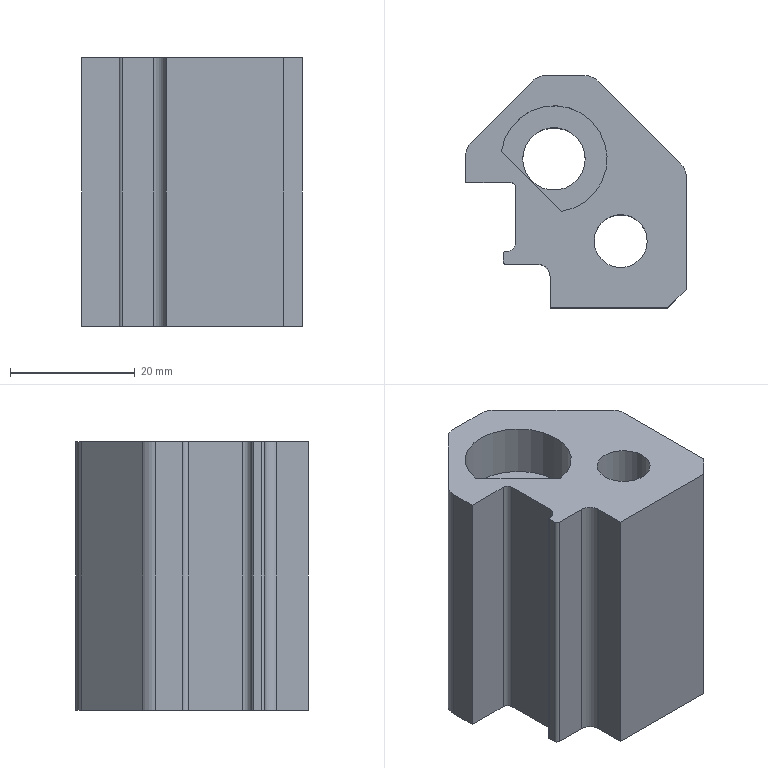Part | NX | features PH-3 2 | 1 solid | 31 faces | box 35.315 x 37.187 x 43 mm | volume 32210 mm3 | plane 18 | cylinder 13 | commonest cylinder face diameters 6 x4 0.6 x1 1 x1 2 x1 3 x1 4 x1
STEP:
#1=CARTESIAN_POINT('',(2388.447,-916.264,902.716));
#2=VERTEX_POINT('',#1);
#3=CARTESIAN_POINT('',(2398.248,-906.463,902.716));
#4=VERTEX_POINT('',#3);
#5=CARTESIAN_POINT('',(2389.755,-914.956,902.716));
#6=DIRECTION('',(-0.7071,-0.7071,0.));
#7=VECTOR('',#6,1000.);
#8=LINE('',#5,#7);
#9=EDGE_CURVE('',#2,#4,#8,.F.);
#10=ORIENTED_EDGE('',*,*,#9,.F.);
#11=CARTESIAN_POINT('',(2388.447,-916.264,945.716));
#12=VERTEX_POINT('',#11);
#13=CARTESIAN_POINT('',(2388.447,-916.264,920.716));
#14=DIRECTION('',(0.,0.,1.));
#15=VECTOR('',#14,1000.);
#16=LINE('',#13,#15);
#17=EDGE_CURVE('',#2,#12,#16,.T.);
#18=ORIENTED_EDGE('',*,*,#17,.T.);
#19=CARTESIAN_POINT('',(2398.248,-906.463,945.716));
#20=VERTEX_POINT('',#19);
#21=CARTESIAN_POINT('',(2389.755,-914.956,945.716));
#22=DIRECTION('',(0.7071,0.7071,0.));
#23=VECTOR('',#22,1000.);
#24=LINE('',#21,#23);
#25=EDGE_CURVE('',#20,#12,#24,.F.);
#26=ORIENTED_EDGE('',*,*,#25,.F.);
#27=CARTESIAN_POINT('',(2398.248,-906.463,920.716));
#28=DIRECTION('',(0.,0.,1.));
#29=VECTOR('',#28,1000.);
#30=LINE('',#27,#29);
#31=EDGE_CURVE('',#20,#4,#30,.F.);
#32=ORIENTED_EDGE('',*,*,#31,.T.);
#33=EDGE_LOOP('',(#10,#18,#26,#32));
#34=FACE_BOUND('',#33,.T.);
#35=CARTESIAN_POINT('',(2397.005,-907.706,920.716));
#36=DIRECTION('',(0.7071,-0.7071,0.));
#37=DIRECTION('',(0.,0.,1.));
#38=AXIS2_PLACEMENT_3D('',#35,#36,#37);
#39=PLANE('',#38);
#40=ADVANCED_FACE('',(#34),#39,.F.);
#41=CARTESIAN_POINT('',(2393.285,-917.695,945.716));
#42=VERTEX_POINT('',#41);
#43=CARTESIAN_POINT('',(2402.901,-927.312,945.716));
#44=VERTEX_POINT('',#43);
#45=CARTESIAN_POINT('',(2398.093,-922.503,945.716));
#46=DIRECTION('',(0.7071,-0.7071,0.));
#47=VECTOR('',#46,1000.);
#48=LINE('',#45,#47);
#49=EDGE_CURVE('',#42,#44,#48,.T.);
#50=ORIENTED_EDGE('',*,*,#49,.F.);
#51=CARTESIAN_POINT('',(2401.699,-918.897,945.716));
#52=DIRECTION('',(0.,0.,-1.));
#53=DIRECTION('',(1.,0.,0.));
#54=AXIS2_PLACEMENT_3D('',#51,#52,#53);
#55=CIRCLE('',#54,8.5);
#56=EDGE_CURVE('',#42,#44,#55,.T.);
#57=ORIENTED_EDGE('',*,*,#56,.T.);
#58=EDGE_LOOP('',(#50,#57));
#59=FACE_BOUND('',#58,.T.);
#60=CARTESIAN_POINT('',(2416.634,-932.085,945.716));
#61=VERTEX_POINT('',#60);
#62=CARTESIAN_POINT('',(2412.384,-932.085,945.716));
#63=DIRECTION('',(0.,0.,1.));
#64=DIRECTION('',(1.,0.,0.));
#65=AXIS2_PLACEMENT_3D('',#62,#63,#64);
#66=CIRCLE('',#65,4.25);
#67=EDGE_CURVE('',#61,#61,#66,.T.);
#68=ORIENTED_EDGE('',*,*,#67,.F.);
#69=EDGE_LOOP('',(#68));
#70=FACE_BOUND('',#69,.T.);
#71=ORIENTED_EDGE('',*,*,#25,.T.);
#72=CARTESIAN_POINT('',(2387.569,-918.385,945.716));
#73=VERTEX_POINT('',#72);
#74=CARTESIAN_POINT('',(2390.569,-918.385,945.716));
#75=DIRECTION('',(0.,0.,1.));
#76=DIRECTION('',(1.,0.,0.));
#77=AXIS2_PLACEMENT_3D('',#74,#75,#76);
#78=CIRCLE('',#77,3.);
#79=EDGE_CURVE('',#12,#73,#78,.T.);
#80=ORIENTED_EDGE('',*,*,#79,.T.);
#81=CARTESIAN_POINT('',(2387.569,-922.622,945.716));
#82=VERTEX_POINT('',#81);
#83=CARTESIAN_POINT('',(2387.569,-923.085,945.716));
#84=DIRECTION('',(0.,-1.,0.));
#85=VECTOR('',#84,1000.);
#86=LINE('',#83,#85);
#87=EDGE_CURVE('',#82,#73,#86,.F.);
#88=ORIENTED_EDGE('',*,*,#87,.F.);
#89=CARTESIAN_POINT('',(2394.569,-922.622,945.716));
#90=VERTEX_POINT('',#89);
#91=CARTESIAN_POINT('',(2393.069,-922.622,945.716));
#92=DIRECTION('',(-1.,0.,0.));
#93=VECTOR('',#92,1000.);
#94=LINE('',#91,#93);
#95=EDGE_CURVE('',#90,#82,#94,.T.);
#96=ORIENTED_EDGE('',*,*,#95,.F.);
#97=CARTESIAN_POINT('',(2395.569,-923.622,945.716));
#98=VERTEX_POINT('',#97);
#99=CARTESIAN_POINT('',(2394.569,-923.622,945.716));
#100=DIRECTION('',(0.,0.,1.));
#101=DIRECTION('',(1.,0.,0.));
#102=AXIS2_PLACEMENT_3D('',#99,#100,#101);
#103=CIRCLE('',#102,1.);
#104=EDGE_CURVE('',#98,#90,#103,.T.);
#105=ORIENTED_EDGE('',*,*,#104,.F.);
#106=CARTESIAN_POINT('',(2395.569,-932.272,945.716));
#107=VERTEX_POINT('',#106);
#108=CARTESIAN_POINT('',(2395.569,-923.085,945.716));
#109=DIRECTION('',(0.,-1.,0.));
#110=VECTOR('',#109,1000.);
#111=LINE('',#108,#110);
#112=EDGE_CURVE('',#107,#98,#111,.F.);
#113=ORIENTED_EDGE('',*,*,#112,.F.);
#114=CARTESIAN_POINT('',(2394.069,-933.772,945.716));
#115=VERTEX_POINT('',#114);
#116=CARTESIAN_POINT('',(2394.069,-932.272,945.716));
#117=DIRECTION('',(0.,0.,1.));
#118=DIRECTION('',(1.,0.,0.));
#119=AXIS2_PLACEMENT_3D('',#116,#117,#118);
#120=CIRCLE('',#119,1.5);
#121=EDGE_CURVE('',#115,#107,#120,.T.);
#122=ORIENTED_EDGE('',*,*,#121,.F.);
#123=CARTESIAN_POINT('',(2393.869,-933.772,945.716));
#124=VERTEX_POINT('',#123);
#125=CARTESIAN_POINT('',(2388.419,-933.772,945.716));
#126=DIRECTION('',(1.,0.,0.));
#127=VECTOR('',#126,1000.);
#128=LINE('',#125,#127);
#129=EDGE_CURVE('',#115,#124,#128,.F.);
#130=ORIENTED_EDGE('',*,*,#129,.T.);
#131=CARTESIAN_POINT('',(2393.569,-934.072,945.716));
#132=VERTEX_POINT('',#131);
#133=CARTESIAN_POINT('',(2393.869,-934.072,945.716));
#134=DIRECTION('',(0.,0.,1.));
#135=DIRECTION('',(1.,0.,0.));
#136=AXIS2_PLACEMENT_3D('',#133,#134,#135);
#137=CIRCLE('',#136,0.3);
#138=EDGE_CURVE('',#132,#124,#137,.F.);
#139=ORIENTED_EDGE('',*,*,#138,.F.);
#140=CARTESIAN_POINT('',(2393.569,-935.272,945.716));
#141=VERTEX_POINT('',#140);
#142=CARTESIAN_POINT('',(2393.569,-933.722,945.716));
#143=DIRECTION('',(0.,-1.,0.));
#144=VECTOR('',#143,1000.);
#145=LINE('',#142,#144);
#146=EDGE_CURVE('',#132,#141,#145,.T.);
#147=ORIENTED_EDGE('',*,*,#146,.T.);
#148=CARTESIAN_POINT('',(2394.069,-935.772,945.716));
#149=VERTEX_POINT('',#148);
#150=CARTESIAN_POINT('',(2394.069,-935.272,945.716));
#151=DIRECTION('',(0.,0.,-1.));
#152=DIRECTION('',(-1.,0.,0.));
#153=AXIS2_PLACEMENT_3D('',#150,#151,#152);
#154=CIRCLE('',#153,0.5);
#155=EDGE_CURVE('',#141,#149,#154,.F.);
#156=ORIENTED_EDGE('',*,*,#155,.T.);
#157=CARTESIAN_POINT('',(2399.069,-935.772,945.716));
#158=VERTEX_POINT('',#157);
#159=CARTESIAN_POINT('',(2475.144,-935.772,945.716));
#160=DIRECTION('',(1.,0.,0.));
#161=VECTOR('',#160,1000.);
#162=LINE('',#159,#161);
#163=EDGE_CURVE('',#149,#158,#162,.T.);
#164=ORIENTED_EDGE('',*,*,#163,.T.);
#165=CARTESIAN_POINT('',(2401.069,-937.772,945.716));
#166=VERTEX_POINT('',#165);
#167=CARTESIAN_POINT('',(2399.069,-937.772,945.716));
#168=DIRECTION('',(0.,0.,-1.));
#169=DIRECTION('',(-1.,0.,0.));
#170=AXIS2_PLACEMENT_3D('',#167,#168,#169);
#171=CIRCLE('',#170,2.);
#172=EDGE_CURVE('',#158,#166,#171,.T.);
#173=ORIENTED_EDGE('',*,*,#172,.T.);
#174=CARTESIAN_POINT('',(2401.069,-942.772,945.716));
#175=VERTEX_POINT('',#174);
#176=CARTESIAN_POINT('',(2401.069,-923.085,945.716));
#177=DIRECTION('',(0.,-1.,0.));
#178=VECTOR('',#177,1000.);
#179=LINE('',#176,#178);
#180=EDGE_CURVE('',#175,#166,#179,.F.);
#181=ORIENTED_EDGE('',*,*,#180,.F.);
#182=CARTESIAN_POINT('',(2419.884,-942.772,945.716));
#183=VERTEX_POINT('',#182);
#184=CARTESIAN_POINT('',(2401.644,-942.772,945.716));
#185=DIRECTION('',(1.,0.,0.));
#186=VECTOR('',#185,1000.);
#187=LINE('',#184,#186);
#188=EDGE_CURVE('',#183,#175,#187,.F.);
#189=ORIENTED_EDGE('',*,*,#188,.F.);
#190=CARTESIAN_POINT('',(2422.884,-939.772,945.716));
#191=VERTEX_POINT('',#190);
#192=CARTESIAN_POINT('',(2418.728,-943.928,945.716));
#193=DIRECTION('',(0.7071,0.7071,0.));
#194=VECTOR('',#193,1000.);
#195=LINE('',#192,#194);
#196=EDGE_CURVE('',#183,#191,#195,.T.);
#197=ORIENTED_EDGE('',*,*,#196,.T.);
#198=CARTESIAN_POINT('',(2422.884,-921.827,945.716));
#199=VERTEX_POINT('',#198);
#200=CARTESIAN_POINT('',(2422.884,-923.085,945.716));
#201=DIRECTION('',(0.,-1.,0.));
#202=VECTOR('',#201,1000.);
#203=LINE('',#200,#202);
#204=EDGE_CURVE('',#199,#191,#203,.T.);
#205=ORIENTED_EDGE('',*,*,#204,.F.);
#206=CARTESIAN_POINT('',(2422.005,-919.706,945.716));
#207=VERTEX_POINT('',#206);
#208=CARTESIAN_POINT('',(2419.884,-921.827,945.716));
#209=DIRECTION('',(0.,0.,1.));
#210=DIRECTION('',(1.,0.,0.));
#211=AXIS2_PLACEMENT_3D('',#208,#209,#210);
#212=CIRCLE('',#211,3.);
#213=EDGE_CURVE('',#199,#207,#212,.T.);
#214=ORIENTED_EDGE('',*,*,#213,.T.);
#215=CARTESIAN_POINT('',(2408.763,-906.463,945.716));
#216=VERTEX_POINT('',#215);
#217=CARTESIAN_POINT('',(2411.634,-909.335,945.716));
#218=DIRECTION('',(0.7071,-0.7071,0.));
#219=VECTOR('',#218,1000.);
#220=LINE('',#217,#219);
#221=EDGE_CURVE('',#207,#216,#220,.F.);
#222=ORIENTED_EDGE('',*,*,#221,.T.);
#223=CARTESIAN_POINT('',(2406.641,-905.585,945.716));
#224=VERTEX_POINT('',#223);
#225=CARTESIAN_POINT('',(2406.641,-908.585,945.716));
#226=DIRECTION('',(0.,0.,1.));
#227=DIRECTION('',(1.,0.,0.));
#228=AXIS2_PLACEMENT_3D('',#225,#226,#227);
#229=CIRCLE('',#228,3.);
#230=EDGE_CURVE('',#216,#224,#229,.T.);
#231=ORIENTED_EDGE('',*,*,#230,.T.);
#232=CARTESIAN_POINT('',(2400.369,-905.585,945.716));
#233=VERTEX_POINT('',#232);
#234=CARTESIAN_POINT('',(2397.884,-905.585,945.716));
#235=DIRECTION('',(1.,0.,0.));
#236=VECTOR('',#235,1000.);
#237=LINE('',#234,#236);
#238=EDGE_CURVE('',#233,#224,#237,.T.);
#239=ORIENTED_EDGE('',*,*,#238,.F.);
#240=CARTESIAN_POINT('',(2400.369,-908.585,945.716));
#241=DIRECTION('',(0.,0.,1.));
#242=DIRECTION('',(1.,0.,0.));
#243=AXIS2_PLACEMENT_3D('',#240,#241,#242);
#244=CIRCLE('',#243,3.);
#245=EDGE_CURVE('',#233,#20,#244,.T.);
#246=ORIENTED_EDGE('',*,*,#245,.T.);
#247=EDGE_LOOP('',(#71,#80,#88,#96,#105,#113,#122,#130,#139,#147,#156,#164,#173,#181,#189,#197,#205,#214,#222,#231,#239,#246));
#248=FACE_BOUND('',#247,.T.);
#249=CARTESIAN_POINT('',(2397.884,-923.085,945.716));
#250=DIRECTION('',(0.,0.,1.));
#251=DIRECTION('',(1.,0.,0.));
#252=AXIS2_PLACEMENT_3D('',#249,#250,#251);
#253=PLANE('',#252);
#254=ADVANCED_FACE('',(#59,#70,#248),#253,.T.);
#255=CARTESIAN_POINT('',(2396.699,-918.897,902.716));
#256=VERTEX_POINT('',#255);
#257=CARTESIAN_POINT('',(2401.699,-918.897,902.716));
#258=DIRECTION('',(0.,0.,-1.));
#259=DIRECTION('',(-1.,0.,0.));
#260=AXIS2_PLACEMENT_3D('',#257,#258,#259);
#261=CIRCLE('',#260,5.);
#262=EDGE_CURVE('',#256,#256,#261,.T.);
#263=ORIENTED_EDGE('',*,*,#262,.F.);
#264=EDGE_LOOP('',(#263));
#265=FACE_BOUND('',#264,.T.);
#266=CARTESIAN_POINT('',(2405.134,-932.085,902.716));
#267=VERTEX_POINT('',#266);
#268=CARTESIAN_POINT('',(2412.384,-932.085,902.716));
#269=DIRECTION('',(0.,0.,-1.));
#270=DIRECTION('',(-1.,0.,0.));
#271=AXIS2_PLACEMENT_3D('',#268,#269,#270);
#272=CIRCLE('',#271,7.25);
#273=EDGE_CURVE('',#267,#267,#272,.T.);
#274=ORIENTED_EDGE('',*,*,#273,.F.);
#275=EDGE_LOOP('',(#274));
#276=FACE_BOUND('',#275,.T.);
#277=CARTESIAN_POINT('',(2387.569,-918.385,902.716));
#278=VERTEX_POINT('',#277);
#279=CARTESIAN_POINT('',(2387.569,-922.622,902.716));
#280=VERTEX_POINT('',#279);
#281=CARTESIAN_POINT('',(2387.569,-927.947,902.716));
#282=DIRECTION('',(0.,-1.,0.));
#283=VECTOR('',#282,1000.);
#284=LINE('',#281,#283);
#285=EDGE_CURVE('',#278,#280,#284,.T.);
#286=ORIENTED_EDGE('',*,*,#285,.F.);
#287=CARTESIAN_POINT('',(2390.569,-918.385,902.716));
#288=DIRECTION('',(0.,0.,-1.));
#289=DIRECTION('',(-1.,0.,0.));
#290=AXIS2_PLACEMENT_3D('',#287,#288,#289);
#291=CIRCLE('',#290,3.);
#292=EDGE_CURVE('',#278,#2,#291,.T.);
#293=ORIENTED_EDGE('',*,*,#292,.T.);
#294=ORIENTED_EDGE('',*,*,#9,.T.);
#295=CARTESIAN_POINT('',(2400.369,-905.585,902.716));
#296=VERTEX_POINT('',#295);
#297=CARTESIAN_POINT('',(2400.369,-908.585,902.716));
#298=DIRECTION('',(0.,0.,-1.));
#299=DIRECTION('',(-1.,0.,0.));
#300=AXIS2_PLACEMENT_3D('',#297,#298,#299);
#301=CIRCLE('',#300,3.);
#302=EDGE_CURVE('',#4,#296,#301,.T.);
#303=ORIENTED_EDGE('',*,*,#302,.T.);
#304=CARTESIAN_POINT('',(2406.641,-905.585,902.716));
#305=VERTEX_POINT('',#304);
#306=CARTESIAN_POINT('',(2397.884,-905.585,902.716));
#307=DIRECTION('',(-1.,0.,0.));
#308=VECTOR('',#307,1000.);
#309=LINE('',#306,#308);
#310=EDGE_CURVE('',#305,#296,#309,.T.);
#311=ORIENTED_EDGE('',*,*,#310,.F.);
#312=CARTESIAN_POINT('',(2408.763,-906.463,902.716));
#313=VERTEX_POINT('',#312);
#314=CARTESIAN_POINT('',(2406.641,-908.585,902.716));
#315=DIRECTION('',(0.,0.,-1.));
#316=DIRECTION('',(-1.,0.,0.));
#317=AXIS2_PLACEMENT_3D('',#314,#315,#316);
#318=CIRCLE('',#317,3.);
#319=EDGE_CURVE('',#305,#313,#318,.T.);
#320=ORIENTED_EDGE('',*,*,#319,.T.);
#321=CARTESIAN_POINT('',(2422.005,-919.706,902.716));
#322=VERTEX_POINT('',#321);
#323=CARTESIAN_POINT('',(2411.634,-909.335,902.716));
#324=DIRECTION('',(-0.7071,0.7071,0.));
#325=VECTOR('',#324,1000.);
#326=LINE('',#323,#325);
#327=EDGE_CURVE('',#313,#322,#326,.F.);
#328=ORIENTED_EDGE('',*,*,#327,.T.);
#329=CARTESIAN_POINT('',(2422.884,-921.827,902.716));
#330=VERTEX_POINT('',#329);
#331=CARTESIAN_POINT('',(2419.884,-921.827,902.716));
#332=DIRECTION('',(0.,0.,-1.));
#333=DIRECTION('',(-1.,0.,0.));
#334=AXIS2_PLACEMENT_3D('',#331,#332,#333);
#335=CIRCLE('',#334,3.);
#336=EDGE_CURVE('',#322,#330,#335,.T.);
#337=ORIENTED_EDGE('',*,*,#336,.T.);
#338=CARTESIAN_POINT('',(2422.884,-939.772,902.716));
#339=VERTEX_POINT('',#338);
#340=CARTESIAN_POINT('',(2422.884,-923.085,902.716));
#341=DIRECTION('',(0.,1.,0.));
#342=VECTOR('',#341,1000.);
#343=LINE('',#340,#342);
#344=EDGE_CURVE('',#339,#330,#343,.T.);
#345=ORIENTED_EDGE('',*,*,#344,.F.);
#346=CARTESIAN_POINT('',(2419.884,-942.772,902.716));
#347=VERTEX_POINT('',#346);
#348=CARTESIAN_POINT('',(2418.728,-943.928,902.716));
#349=DIRECTION('',(-0.7071,-0.7071,0.));
#350=VECTOR('',#349,1000.);
#351=LINE('',#348,#350);
#352=EDGE_CURVE('',#339,#347,#351,.T.);
#353=ORIENTED_EDGE('',*,*,#352,.T.);
#354=CARTESIAN_POINT('',(2401.069,-942.772,902.716));
#355=VERTEX_POINT('',#354);
#356=CARTESIAN_POINT('',(2401.644,-942.772,902.716));
#357=DIRECTION('',(-1.,0.,0.));
#358=VECTOR('',#357,1000.);
#359=LINE('',#356,#358);
#360=EDGE_CURVE('',#355,#347,#359,.F.);
#361=ORIENTED_EDGE('',*,*,#360,.F.);
#362=CARTESIAN_POINT('',(2401.069,-937.772,902.716));
#363=VERTEX_POINT('',#362);
#364=CARTESIAN_POINT('',(2401.069,-945.272,902.716));
#365=DIRECTION('',(0.,-1.,0.));
#366=VECTOR('',#365,1000.);
#367=LINE('',#364,#366);
#368=EDGE_CURVE('',#363,#355,#367,.T.);
#369=ORIENTED_EDGE('',*,*,#368,.F.);
#370=CARTESIAN_POINT('',(2399.069,-935.772,902.716));
#371=VERTEX_POINT('',#370);
#372=CARTESIAN_POINT('',(2399.069,-937.772,902.716));
#373=DIRECTION('',(0.,0.,-1.));
#374=DIRECTION('',(-1.,0.,0.));
#375=AXIS2_PLACEMENT_3D('',#372,#373,#374);
#376=CIRCLE('',#375,2.);
#377=EDGE_CURVE('',#371,#363,#376,.T.);
#378=ORIENTED_EDGE('',*,*,#377,.F.);
#379=CARTESIAN_POINT('',(2394.069,-935.772,902.716));
#380=VERTEX_POINT('',#379);
#381=CARTESIAN_POINT('',(2397.884,-935.772,902.716));
#382=DIRECTION('',(1.,0.,0.));
#383=VECTOR('',#382,1000.);
#384=LINE('',#381,#383);
#385=EDGE_CURVE('',#380,#371,#384,.T.);
#386=ORIENTED_EDGE('',*,*,#385,.F.);
#387=CARTESIAN_POINT('',(2393.569,-935.272,902.716));
#388=VERTEX_POINT('',#387);
#389=CARTESIAN_POINT('',(2394.069,-935.272,902.716));
#390=DIRECTION('',(0.,0.,-1.));
#391=DIRECTION('',(-1.,0.,0.));
#392=AXIS2_PLACEMENT_3D('',#389,#390,#391);
#393=CIRCLE('',#392,0.5);
#394=EDGE_CURVE('',#380,#388,#393,.T.);
#395=ORIENTED_EDGE('',*,*,#394,.T.);
#396=CARTESIAN_POINT('',(2393.569,-934.072,902.716));
#397=VERTEX_POINT('',#396);
#398=CARTESIAN_POINT('',(2393.569,-923.085,902.716));
#399=DIRECTION('',(0.,1.,0.));
#400=VECTOR('',#399,1000.);
#401=LINE('',#398,#400);
#402=EDGE_CURVE('',#388,#397,#401,.T.);
#403=ORIENTED_EDGE('',*,*,#402,.T.);
#404=CARTESIAN_POINT('',(2393.869,-933.772,902.716));
#405=VERTEX_POINT('',#404);
#406=CARTESIAN_POINT('',(2393.869,-934.072,902.716));
#407=DIRECTION('',(0.,0.,-1.));
#408=DIRECTION('',(-1.,0.,0.));
#409=AXIS2_PLACEMENT_3D('',#406,#407,#408);
#410=CIRCLE('',#409,0.3);
#411=EDGE_CURVE('',#397,#405,#410,.T.);
#412=ORIENTED_EDGE('',*,*,#411,.T.);
#413=CARTESIAN_POINT('',(2394.069,-933.772,902.716));
#414=VERTEX_POINT('',#413);
#415=CARTESIAN_POINT('',(2397.884,-933.772,902.716));
#416=DIRECTION('',(1.,0.,0.));
#417=VECTOR('',#416,1000.);
#418=LINE('',#415,#417);
#419=EDGE_CURVE('',#405,#414,#418,.T.);
#420=ORIENTED_EDGE('',*,*,#419,.T.);
#421=CARTESIAN_POINT('',(2395.569,-932.272,902.716));
#422=VERTEX_POINT('',#421);
#423=CARTESIAN_POINT('',(2394.069,-932.272,902.716));
#424=DIRECTION('',(0.,0.,-1.));
#425=DIRECTION('',(-1.,0.,0.));
#426=AXIS2_PLACEMENT_3D('',#423,#424,#425);
#427=CIRCLE('',#426,1.5);
#428=EDGE_CURVE('',#422,#414,#427,.T.);
#429=ORIENTED_EDGE('',*,*,#428,.F.);
#430=CARTESIAN_POINT('',(2395.569,-923.622,902.716));
#431=VERTEX_POINT('',#430);
#432=CARTESIAN_POINT('',(2395.569,-923.085,902.716));
#433=DIRECTION('',(0.,1.,0.));
#434=VECTOR('',#433,1000.);
#435=LINE('',#432,#434);
#436=EDGE_CURVE('',#422,#431,#435,.T.);
#437=ORIENTED_EDGE('',*,*,#436,.T.);
#438=CARTESIAN_POINT('',(2394.569,-922.622,902.716));
#439=VERTEX_POINT('',#438);
#440=CARTESIAN_POINT('',(2394.569,-923.622,902.716));
#441=DIRECTION('',(0.,0.,-1.));
#442=DIRECTION('',(-1.,0.,0.));
#443=AXIS2_PLACEMENT_3D('',#440,#441,#442);
#444=CIRCLE('',#443,1.);
#445=EDGE_CURVE('',#439,#431,#444,.T.);
#446=ORIENTED_EDGE('',*,*,#445,.F.);
#447=CARTESIAN_POINT('',(2393.069,-922.622,902.716));
#448=DIRECTION('',(1.,0.,0.));
#449=VECTOR('',#448,1000.);
#450=LINE('',#447,#449);
#451=EDGE_CURVE('',#280,#439,#450,.T.);
#452=ORIENTED_EDGE('',*,*,#451,.F.);
#453=EDGE_LOOP('',(#286,#293,#294,#303,#311,#320,#328,#337,#345,#353,#361,#369,#378,#386,#395,#403,#412,#420,#429,#437,#446,#452));
#454=FACE_BOUND('',#453,.T.);
#455=CARTESIAN_POINT('',(2397.884,-923.085,902.716));
#456=DIRECTION('',(0.,0.,-1.));
#457=DIRECTION('',(-1.,0.,0.));
#458=AXIS2_PLACEMENT_3D('',#455,#456,#457);
#459=PLANE('',#458);
#460=ADVANCED_FACE('',(#265,#276,#454),#459,.T.);
#461=ORIENTED_EDGE('',*,*,#95,.T.);
#462=CARTESIAN_POINT('',(2387.569,-922.622,950.716));
#463=DIRECTION('',(0.,0.,-1.));
#464=VECTOR('',#463,1000.);
#465=LINE('',#462,#464);
#466=EDGE_CURVE('',#82,#280,#465,.T.);
#467=ORIENTED_EDGE('',*,*,#466,.T.);
#468=ORIENTED_EDGE('',*,*,#451,.T.);
#469=CARTESIAN_POINT('',(2394.569,-922.622,950.716));
#470=DIRECTION('',(0.,0.,-1.));
#471=VECTOR('',#470,1000.);
#472=LINE('',#469,#471);
#473=EDGE_CURVE('',#90,#439,#472,.T.);
#474=ORIENTED_EDGE('',*,*,#473,.F.);
#475=EDGE_LOOP('',(#461,#467,#468,#474));
#476=FACE_BOUND('',#475,.T.);
#477=CARTESIAN_POINT('',(2393.069,-922.622,950.716));
#478=DIRECTION('',(0.,-1.,0.));
#479=DIRECTION('',(0.,0.,1.));
#480=AXIS2_PLACEMENT_3D('',#477,#478,#479);
#481=PLANE('',#480);
#482=ADVANCED_FACE('',(#476),#481,.T.);
#483=ORIENTED_EDGE('',*,*,#310,.T.);
#484=CARTESIAN_POINT('',(2400.369,-905.585,920.716));
#485=DIRECTION('',(0.,0.,-1.));
#486=VECTOR('',#485,1000.);
#487=LINE('',#484,#486);
#488=EDGE_CURVE('',#296,#233,#487,.F.);
#489=ORIENTED_EDGE('',*,*,#488,.T.);
#490=ORIENTED_EDGE('',*,*,#238,.T.);
#491=CARTESIAN_POINT('',(2406.641,-905.585,920.716));
#492=DIRECTION('',(0.,0.,1.));
#493=VECTOR('',#492,1000.);
#494=LINE('',#491,#493);
#495=EDGE_CURVE('',#224,#305,#494,.F.);
#496=ORIENTED_EDGE('',*,*,#495,.T.);
#497=EDGE_LOOP('',(#483,#489,#490,#496));
#498=FACE_BOUND('',#497,.T.);
#499=CARTESIAN_POINT('',(2397.884,-905.585,920.716));
#500=DIRECTION('',(0.,1.,0.));
#501=DIRECTION('',(0.,0.,1.));
#502=AXIS2_PLACEMENT_3D('',#499,#500,#501);
#503=PLANE('',#502);
#504=ADVANCED_FACE('',(#498),#503,.T.);
#505=ORIENTED_EDGE('',*,*,#344,.T.);
#506=CARTESIAN_POINT('',(2422.884,-921.827,920.716));
#507=DIRECTION('',(0.,0.,-1.));
#508=VECTOR('',#507,1000.);
#509=LINE('',#506,#508);
#510=EDGE_CURVE('',#330,#199,#509,.F.);
#511=ORIENTED_EDGE('',*,*,#510,.T.);
#512=ORIENTED_EDGE('',*,*,#204,.T.);
#513=CARTESIAN_POINT('',(2422.884,-939.772,920.716));
#514=DIRECTION('',(0.,0.,-1.));
#515=VECTOR('',#514,1000.);
#516=LINE('',#513,#515);
#517=EDGE_CURVE('',#191,#339,#516,.T.);
#518=ORIENTED_EDGE('',*,*,#517,.T.);
#519=EDGE_LOOP('',(#505,#511,#512,#518));
#520=FACE_BOUND('',#519,.T.);
#521=CARTESIAN_POINT('',(2422.884,-923.085,920.716));
#522=DIRECTION('',(1.,0.,0.));
#523=DIRECTION('',(0.,0.,-1.));
#524=AXIS2_PLACEMENT_3D('',#521,#522,#523);
#525=PLANE('',#524);
#526=ADVANCED_FACE('',(#520),#525,.T.);
#527=CARTESIAN_POINT('',(2402.901,-927.312,937.416));
#528=VERTEX_POINT('',#527);
#529=CARTESIAN_POINT('',(2393.285,-917.695,937.416));
#530=VERTEX_POINT('',#529);
#531=CARTESIAN_POINT('',(2398.093,-922.503,937.416));
#532=DIRECTION('',(-0.7071,0.7071,0.));
#533=VECTOR('',#532,1000.);
#534=LINE('',#531,#533);
#535=EDGE_CURVE('',#528,#530,#534,.T.);
#536=ORIENTED_EDGE('',*,*,#535,.F.);
#537=CARTESIAN_POINT('',(2401.699,-918.897,937.416));
#538=DIRECTION('',(0.,0.,1.));
#539=DIRECTION('',(1.,0.,0.));
#540=AXIS2_PLACEMENT_3D('',#537,#538,#539);
#541=CIRCLE('',#540,8.5);
#542=EDGE_CURVE('',#528,#530,#541,.T.);
#543=ORIENTED_EDGE('',*,*,#542,.T.);
#544=EDGE_LOOP('',(#536,#543));
#545=FACE_BOUND('',#544,.T.);
#546=CARTESIAN_POINT('',(2396.699,-918.897,937.416));
#547=VERTEX_POINT('',#546);
#548=CARTESIAN_POINT('',(2401.699,-918.897,937.416));
#549=DIRECTION('',(0.,0.,-1.));
#550=DIRECTION('',(-1.,0.,0.));
#551=AXIS2_PLACEMENT_3D('',#548,#549,#550);
#552=CIRCLE('',#551,5.);
#553=EDGE_CURVE('',#547,#547,#552,.F.);
#554=ORIENTED_EDGE('',*,*,#553,.F.);
#555=EDGE_LOOP('',(#554));
#556=FACE_BOUND('',#555,.T.);
#557=CARTESIAN_POINT('',(2401.699,-918.897,937.416));
#558=DIRECTION('',(0.,0.,-1.));
#559=DIRECTION('',(-1.,0.,0.));
#560=AXIS2_PLACEMENT_3D('',#557,#558,#559);
#561=PLANE('',#560);
#562=ADVANCED_FACE('',(#545,#556),#561,.F.);
#563=CARTESIAN_POINT('',(2393.869,-933.772,874.217));
#564=DIRECTION('',(0.,0.,-1.));
#565=VECTOR('',#564,1000.);
#566=LINE('',#563,#565);
#567=EDGE_CURVE('',#124,#405,#566,.T.);
#568=ORIENTED_EDGE('',*,*,#567,.F.);
#569=ORIENTED_EDGE('',*,*,#129,.F.);
#570=CARTESIAN_POINT('',(2394.069,-933.772,950.716));
#571=DIRECTION('',(0.,0.,1.));
#572=VECTOR('',#571,1000.);
#573=LINE('',#570,#572);
#574=EDGE_CURVE('',#115,#414,#573,.F.);
#575=ORIENTED_EDGE('',*,*,#574,.T.);
#576=ORIENTED_EDGE('',*,*,#419,.F.);
#577=EDGE_LOOP('',(#568,#569,#575,#576));
#578=FACE_BOUND('',#577,.T.);
#579=CARTESIAN_POINT('',(2388.419,-933.772,950.716));
#580=DIRECTION('',(0.,1.,0.));
#581=DIRECTION('',(0.,0.,-1.));
#582=AXIS2_PLACEMENT_3D('',#579,#580,#581);
#583=PLANE('',#582);
#584=ADVANCED_FACE('',(#578),#583,.T.);
#585=ORIENTED_EDGE('',*,*,#112,.T.);
#586=CARTESIAN_POINT('',(2395.569,-923.622,950.716));
#587=DIRECTION('',(0.,0.,-1.));
#588=VECTOR('',#587,1000.);
#589=LINE('',#586,#588);
#590=EDGE_CURVE('',#431,#98,#589,.F.);
#591=ORIENTED_EDGE('',*,*,#590,.F.);
#592=ORIENTED_EDGE('',*,*,#436,.F.);
#593=CARTESIAN_POINT('',(2395.569,-932.272,950.716));
#594=DIRECTION('',(0.,0.,-1.));
#595=VECTOR('',#594,1000.);
#596=LINE('',#593,#595);
#597=EDGE_CURVE('',#422,#107,#596,.F.);
#598=ORIENTED_EDGE('',*,*,#597,.T.);
#599=EDGE_LOOP('',(#585,#591,#592,#598));
#600=FACE_BOUND('',#599,.T.);
#601=CARTESIAN_POINT('',(2395.569,-932.772,950.716));
#602=DIRECTION('',(-1.,0.,0.));
#603=DIRECTION('',(0.,0.,-1.));
#604=AXIS2_PLACEMENT_3D('',#601,#602,#603);
#605=PLANE('',#604);
#606=ADVANCED_FACE('',(#600),#605,.T.);
#607=ORIENTED_EDGE('',*,*,#590,.T.);
#608=ORIENTED_EDGE('',*,*,#104,.T.);
#609=ORIENTED_EDGE('',*,*,#473,.T.);
#610=ORIENTED_EDGE('',*,*,#445,.T.);
#611=EDGE_LOOP('',(#607,#608,#609,#610));
#612=FACE_BOUND('',#611,.T.);
#613=CARTESIAN_POINT('',(2394.569,-923.622,950.716));
#614=DIRECTION('',(0.,0.,-1.));
#615=DIRECTION('',(1.,0.,0.));
#616=AXIS2_PLACEMENT_3D('',#613,#614,#615);
#617=CYLINDRICAL_SURFACE('',#616,1.);
#618=ADVANCED_FACE('',(#612),#617,.F.);
#619=ORIENTED_EDGE('',*,*,#574,.F.);
#620=ORIENTED_EDGE('',*,*,#121,.T.);
#621=ORIENTED_EDGE('',*,*,#597,.F.);
#622=ORIENTED_EDGE('',*,*,#428,.T.);
#623=EDGE_LOOP('',(#619,#620,#621,#622));
#624=FACE_BOUND('',#623,.T.);
#625=CARTESIAN_POINT('',(2394.069,-932.272,950.716));
#626=DIRECTION('',(0.,0.,-1.));
#627=DIRECTION('',(1.,0.,0.));
#628=AXIS2_PLACEMENT_3D('',#625,#626,#627);
#629=CYLINDRICAL_SURFACE('',#628,1.5);
#630=ADVANCED_FACE('',(#624),#629,.F.);
#631=CARTESIAN_POINT('',(2393.569,-934.072,945.716));
#632=DIRECTION('',(0.,0.,-1.));
#633=VECTOR('',#632,1000.);
#634=LINE('',#631,#633);
#635=EDGE_CURVE('',#132,#397,#634,.T.);
#636=ORIENTED_EDGE('',*,*,#635,.F.);
#637=ORIENTED_EDGE('',*,*,#138,.T.);
#638=ORIENTED_EDGE('',*,*,#567,.T.);
#639=ORIENTED_EDGE('',*,*,#411,.F.);
#640=EDGE_LOOP('',(#636,#637,#638,#639));
#641=FACE_BOUND('',#640,.T.);
#642=CARTESIAN_POINT('',(2393.869,-934.072,940.716));
#643=DIRECTION('',(0.,0.,1.));
#644=DIRECTION('',(1.,0.,0.));
#645=AXIS2_PLACEMENT_3D('',#642,#643,#644);
#646=CYLINDRICAL_SURFACE('',#645,0.3);
#647=ADVANCED_FACE('',(#641),#646,.T.);
#648=ORIENTED_EDGE('',*,*,#377,.T.);
#649=CARTESIAN_POINT('',(2401.069,-937.772,893.217));
#650=DIRECTION('',(0.,0.,1.));
#651=VECTOR('',#650,1000.);
#652=LINE('',#649,#651);
#653=EDGE_CURVE('',#363,#166,#652,.T.);
#654=ORIENTED_EDGE('',*,*,#653,.T.);
#655=ORIENTED_EDGE('',*,*,#172,.F.);
#656=CARTESIAN_POINT('',(2399.069,-935.772,945.716));
#657=DIRECTION('',(0.,0.,1.));
#658=VECTOR('',#657,1000.);
#659=LINE('',#656,#658);
#660=EDGE_CURVE('',#158,#371,#659,.F.);
#661=ORIENTED_EDGE('',*,*,#660,.T.);
#662=EDGE_LOOP('',(#648,#654,#655,#661));
#663=FACE_BOUND('',#662,.T.);
#664=CARTESIAN_POINT('',(2399.069,-937.772,916.216));
#665=DIRECTION('',(0.,0.,-1.));
#666=DIRECTION('',(1.,0.,0.));
#667=AXIS2_PLACEMENT_3D('',#664,#665,#666);
#668=CYLINDRICAL_SURFACE('',#667,2.);
#669=ADVANCED_FACE('',(#663),#668,.F.);
#670=ORIENTED_EDGE('',*,*,#385,.T.);
#671=ORIENTED_EDGE('',*,*,#660,.F.);
#672=ORIENTED_EDGE('',*,*,#163,.F.);
#673=CARTESIAN_POINT('',(2394.069,-935.772,916.216));
#674=DIRECTION('',(0.,0.,1.));
#675=VECTOR('',#674,1000.);
#676=LINE('',#673,#675);
#677=EDGE_CURVE('',#380,#149,#676,.T.);
#678=ORIENTED_EDGE('',*,*,#677,.F.);
#679=EDGE_LOOP('',(#670,#671,#672,#678));
#680=FACE_BOUND('',#679,.T.);
#681=CARTESIAN_POINT('',(2389.319,-935.772,916.216));
#682=DIRECTION('',(0.,1.,0.));
#683=DIRECTION('',(0.,0.,-1.));
#684=AXIS2_PLACEMENT_3D('',#681,#682,#683);
#685=PLANE('',#684);
#686=ADVANCED_FACE('',(#680),#685,.F.);
#687=ORIENTED_EDGE('',*,*,#677,.T.);
#688=ORIENTED_EDGE('',*,*,#155,.F.);
#689=CARTESIAN_POINT('',(2393.569,-935.272,929.216));
#690=DIRECTION('',(0.,0.,1.));
#691=VECTOR('',#690,1000.);
#692=LINE('',#689,#691);
#693=EDGE_CURVE('',#141,#388,#692,.F.);
#694=ORIENTED_EDGE('',*,*,#693,.T.);
#695=ORIENTED_EDGE('',*,*,#394,.F.);
#696=EDGE_LOOP('',(#687,#688,#694,#695));
#697=FACE_BOUND('',#696,.T.);
#698=CARTESIAN_POINT('',(2394.069,-935.272,929.216));
#699=DIRECTION('',(0.,0.,1.));
#700=DIRECTION('',(-1.,0.,0.));
#701=AXIS2_PLACEMENT_3D('',#698,#699,#700);
#702=CYLINDRICAL_SURFACE('',#701,0.5);
#703=ADVANCED_FACE('',(#697),#702,.T.);
#704=ORIENTED_EDGE('',*,*,#693,.F.);
#705=ORIENTED_EDGE('',*,*,#146,.F.);
#706=ORIENTED_EDGE('',*,*,#635,.T.);
#707=ORIENTED_EDGE('',*,*,#402,.F.);
#708=EDGE_LOOP('',(#704,#705,#706,#707));
#709=FACE_BOUND('',#708,.T.);
#710=CARTESIAN_POINT('',(2393.569,-933.722,929.216));
#711=DIRECTION('',(-1.,0.,0.));
#712=DIRECTION('',(0.,0.,-1.));
#713=AXIS2_PLACEMENT_3D('',#710,#711,#712);
#714=PLANE('',#713);
#715=ADVANCED_FACE('',(#709),#714,.T.);
#716=ORIENTED_EDGE('',*,*,#653,.F.);
#717=ORIENTED_EDGE('',*,*,#368,.T.);
#718=CARTESIAN_POINT('',(2401.069,-942.772,929.216));
#719=DIRECTION('',(0.,0.,1.));
#720=VECTOR('',#719,1000.);
#721=LINE('',#718,#720);
#722=EDGE_CURVE('',#175,#355,#721,.F.);
#723=ORIENTED_EDGE('',*,*,#722,.F.);
#724=ORIENTED_EDGE('',*,*,#180,.T.);
#725=EDGE_LOOP('',(#716,#717,#723,#724));
#726=FACE_BOUND('',#725,.T.);
#727=CARTESIAN_POINT('',(2401.069,-945.272,933.216));
#728=DIRECTION('',(-1.,0.,0.));
#729=DIRECTION('',(0.,0.,1.));
#730=AXIS2_PLACEMENT_3D('',#727,#728,#729);
#731=PLANE('',#730);
#732=ADVANCED_FACE('',(#726),#731,.T.);
#733=ORIENTED_EDGE('',*,*,#352,.F.);
#734=ORIENTED_EDGE('',*,*,#517,.F.);
#735=ORIENTED_EDGE('',*,*,#196,.F.);
#736=CARTESIAN_POINT('',(2419.884,-942.772,929.216));
#737=DIRECTION('',(0.,0.,-1.));
#738=VECTOR('',#737,1000.);
#739=LINE('',#736,#738);
#740=EDGE_CURVE('',#347,#183,#739,.F.);
#741=ORIENTED_EDGE('',*,*,#740,.F.);
#742=EDGE_LOOP('',(#733,#734,#735,#741));
#743=FACE_BOUND('',#742,.T.);
#744=CARTESIAN_POINT('',(2419.884,-942.772,929.216));
#745=DIRECTION('',(0.7071,-0.7071,0.));
#746=DIRECTION('',(0.7071,0.7071,0.));
#747=AXIS2_PLACEMENT_3D('',#744,#745,#746);
#748=PLANE('',#747);
#749=ADVANCED_FACE('',(#743),#748,.T.);
#750=ORIENTED_EDGE('',*,*,#188,.T.);
#751=ORIENTED_EDGE('',*,*,#722,.T.);
#752=ORIENTED_EDGE('',*,*,#360,.T.);
#753=ORIENTED_EDGE('',*,*,#740,.T.);
#754=EDGE_LOOP('',(#750,#751,#752,#753));
#755=FACE_BOUND('',#754,.T.);
#756=CARTESIAN_POINT('',(2401.644,-942.772,929.216));
#757=DIRECTION('',(0.,1.,0.));
#758=DIRECTION('',(0.,0.,1.));
#759=AXIS2_PLACEMENT_3D('',#756,#757,#758);
#760=PLANE('',#759);
#761=ADVANCED_FACE('',(#755),#760,.F.);
#762=ORIENTED_EDGE('',*,*,#87,.T.);
#763=CARTESIAN_POINT('',(2387.569,-918.385,898.966));
#764=DIRECTION('',(0.,0.,-1.));
#765=VECTOR('',#764,1000.);
#766=LINE('',#763,#765);
#767=EDGE_CURVE('',#73,#278,#766,.T.);
#768=ORIENTED_EDGE('',*,*,#767,.T.);
#769=ORIENTED_EDGE('',*,*,#285,.T.);
#770=ORIENTED_EDGE('',*,*,#466,.F.);
#771=EDGE_LOOP('',(#762,#768,#769,#770));
#772=FACE_BOUND('',#771,.T.);
#773=CARTESIAN_POINT('',(2387.569,-927.947,898.966));
#774=DIRECTION('',(-1.,0.,0.));
#775=DIRECTION('',(0.,0.,1.));
#776=AXIS2_PLACEMENT_3D('',#773,#774,#775);
#777=PLANE('',#776);
#778=ADVANCED_FACE('',(#772),#777,.T.);
#779=ORIENTED_EDGE('',*,*,#67,.T.);
#780=EDGE_LOOP('',(#779));
#781=FACE_BOUND('',#780,.T.);
#782=CARTESIAN_POINT('',(2408.134,-932.085,913.716));
#783=VERTEX_POINT('',#782);
#784=CARTESIAN_POINT('',(2412.384,-932.085,913.716));
#785=DIRECTION('',(0.,0.,-1.));
#786=DIRECTION('',(-1.,0.,0.));
#787=AXIS2_PLACEMENT_3D('',#784,#785,#786);
#788=CIRCLE('',#787,4.25);
#789=EDGE_CURVE('',#783,#783,#788,.T.);
#790=ORIENTED_EDGE('',*,*,#789,.T.);
#791=EDGE_LOOP('',(#790));
#792=FACE_BOUND('',#791,.T.);
#793=CARTESIAN_POINT('',(2412.384,-932.085,946.716));
#794=DIRECTION('',(0.,0.,-1.));
#795=DIRECTION('',(-1.,0.,0.));
#796=AXIS2_PLACEMENT_3D('',#793,#794,#795);
#797=CYLINDRICAL_SURFACE('',#796,4.25);
#798=ADVANCED_FACE('',(#781,#792),#797,.F.);
#799=ORIENTED_EDGE('',*,*,#273,.T.);
#800=EDGE_LOOP('',(#799));
#801=FACE_BOUND('',#800,.T.);
#802=CARTESIAN_POINT('',(2405.134,-932.085,913.716));
#803=VERTEX_POINT('',#802);
#804=CARTESIAN_POINT('',(2412.384,-932.085,913.716));
#805=DIRECTION('',(0.,0.,-1.));
#806=DIRECTION('',(-1.,0.,0.));
#807=AXIS2_PLACEMENT_3D('',#804,#805,#806);
#808=CIRCLE('',#807,7.25);
#809=EDGE_CURVE('',#803,#803,#808,.F.);
#810=ORIENTED_EDGE('',*,*,#809,.T.);
#811=EDGE_LOOP('',(#810));
#812=FACE_BOUND('',#811,.T.);
#813=CARTESIAN_POINT('',(2412.384,-932.085,931.716));
#814=DIRECTION('',(0.,0.,-1.));
#815=DIRECTION('',(-1.,0.,0.));
#816=AXIS2_PLACEMENT_3D('',#813,#814,#815);
#817=CYLINDRICAL_SURFACE('',#816,7.25);
#818=ADVANCED_FACE('',(#801,#812),#817,.F.);
#819=ORIENTED_EDGE('',*,*,#789,.F.);
#820=EDGE_LOOP('',(#819));
#821=FACE_BOUND('',#820,.T.);
#822=ORIENTED_EDGE('',*,*,#809,.F.);
#823=EDGE_LOOP('',(#822));
#824=FACE_BOUND('',#823,.T.);
#825=CARTESIAN_POINT('',(2412.384,-932.085,913.716));
#826=DIRECTION('',(0.,0.,-1.));
#827=DIRECTION('',(-1.,0.,0.));
#828=AXIS2_PLACEMENT_3D('',#825,#826,#827);
#829=PLANE('',#828);
#830=ADVANCED_FACE('',(#821,#824),#829,.T.);
#831=ORIENTED_EDGE('',*,*,#221,.F.);
#832=CARTESIAN_POINT('',(2422.005,-919.706,920.716));
#833=DIRECTION('',(0.,0.,1.));
#834=VECTOR('',#833,1000.);
#835=LINE('',#832,#834);
#836=EDGE_CURVE('',#207,#322,#835,.F.);
#837=ORIENTED_EDGE('',*,*,#836,.T.);
#838=ORIENTED_EDGE('',*,*,#327,.F.);
#839=CARTESIAN_POINT('',(2408.763,-906.463,920.716));
#840=DIRECTION('',(0.,0.,-1.));
#841=VECTOR('',#840,1000.);
#842=LINE('',#839,#841);
#843=EDGE_CURVE('',#313,#216,#842,.F.);
#844=ORIENTED_EDGE('',*,*,#843,.T.);
#845=EDGE_LOOP('',(#831,#837,#838,#844));
#846=FACE_BOUND('',#845,.T.);
#847=CARTESIAN_POINT('',(2422.884,-920.585,920.716));
#848=DIRECTION('',(-0.7071,-0.7071,0.));
#849=DIRECTION('',(0.,0.,1.));
#850=AXIS2_PLACEMENT_3D('',#847,#848,#849);
#851=PLANE('',#850);
#852=ADVANCED_FACE('',(#846),#851,.F.);
#853=ORIENTED_EDGE('',*,*,#336,.F.);
#854=ORIENTED_EDGE('',*,*,#836,.F.);
#855=ORIENTED_EDGE('',*,*,#213,.F.);
#856=ORIENTED_EDGE('',*,*,#510,.F.);
#857=EDGE_LOOP('',(#853,#854,#855,#856));
#858=FACE_BOUND('',#857,.T.);
#859=CARTESIAN_POINT('',(2419.884,-921.827,920.716));
#860=DIRECTION('',(0.,0.,-1.));
#861=DIRECTION('',(-1.,0.,0.));
#862=AXIS2_PLACEMENT_3D('',#859,#860,#861);
#863=CYLINDRICAL_SURFACE('',#862,3.);
#864=ADVANCED_FACE('',(#858),#863,.T.);
#865=ORIENTED_EDGE('',*,*,#230,.F.);
#866=ORIENTED_EDGE('',*,*,#843,.F.);
#867=ORIENTED_EDGE('',*,*,#319,.F.);
#868=ORIENTED_EDGE('',*,*,#495,.F.);
#869=EDGE_LOOP('',(#865,#866,#867,#868));
#870=FACE_BOUND('',#869,.T.);
#871=CARTESIAN_POINT('',(2406.641,-908.585,920.716));
#872=DIRECTION('',(0.,0.,1.));
#873=DIRECTION('',(1.,0.,0.));
#874=AXIS2_PLACEMENT_3D('',#871,#872,#873);
#875=CYLINDRICAL_SURFACE('',#874,3.);
#876=ADVANCED_FACE('',(#870),#875,.T.);
#877=ORIENTED_EDGE('',*,*,#302,.F.);
#878=ORIENTED_EDGE('',*,*,#31,.F.);
#879=ORIENTED_EDGE('',*,*,#245,.F.);
#880=ORIENTED_EDGE('',*,*,#488,.F.);
#881=EDGE_LOOP('',(#877,#878,#879,#880));
#882=FACE_BOUND('',#881,.T.);
#883=CARTESIAN_POINT('',(2400.369,-908.585,920.716));
#884=DIRECTION('',(0.,0.,-1.));
#885=DIRECTION('',(-1.,0.,0.));
#886=AXIS2_PLACEMENT_3D('',#883,#884,#885);
#887=CYLINDRICAL_SURFACE('',#886,3.);
#888=ADVANCED_FACE('',(#882),#887,.T.);
#889=ORIENTED_EDGE('',*,*,#292,.F.);
#890=ORIENTED_EDGE('',*,*,#767,.F.);
#891=ORIENTED_EDGE('',*,*,#79,.F.);
#892=ORIENTED_EDGE('',*,*,#17,.F.);
#893=EDGE_LOOP('',(#889,#890,#891,#892));
#894=FACE_BOUND('',#893,.T.);
#895=CARTESIAN_POINT('',(2390.569,-918.385,920.716));
#896=DIRECTION('',(0.,0.,-1.));
#897=DIRECTION('',(-1.,0.,0.));
#898=AXIS2_PLACEMENT_3D('',#895,#896,#897);
#899=CYLINDRICAL_SURFACE('',#898,3.);
#900=ADVANCED_FACE('',(#894),#899,.T.);
#901=ORIENTED_EDGE('',*,*,#49,.T.);
#902=CARTESIAN_POINT('',(2402.901,-927.312,945.716));
#903=DIRECTION('',(0.,0.,-1.));
#904=VECTOR('',#903,1000.);
#905=LINE('',#902,#904);
#906=EDGE_CURVE('',#528,#44,#905,.F.);
#907=ORIENTED_EDGE('',*,*,#906,.F.);
#908=ORIENTED_EDGE('',*,*,#535,.T.);
#909=CARTESIAN_POINT('',(2393.285,-917.695,945.716));
#910=DIRECTION('',(0.,0.,-1.));
#911=VECTOR('',#910,1000.);
#912=LINE('',#909,#911);
#913=EDGE_CURVE('',#42,#530,#912,.T.);
#914=ORIENTED_EDGE('',*,*,#913,.F.);
#915=EDGE_LOOP('',(#901,#907,#908,#914));
#916=FACE_BOUND('',#915,.T.);
#917=CARTESIAN_POINT('',(2398.093,-922.503,960.966));
#918=DIRECTION('',(-0.7071,-0.7071,0.));
#919=DIRECTION('',(0.7071,-0.7071,0.));
#920=AXIS2_PLACEMENT_3D('',#917,#918,#919);
#921=PLANE('',#920);
#922=ADVANCED_FACE('',(#916),#921,.F.);
#923=ORIENTED_EDGE('',*,*,#542,.F.);
#924=ORIENTED_EDGE('',*,*,#906,.T.);
#925=ORIENTED_EDGE('',*,*,#56,.F.);
#926=ORIENTED_EDGE('',*,*,#913,.T.);
#927=EDGE_LOOP('',(#923,#924,#925,#926));
#928=FACE_BOUND('',#927,.T.);
#929=CARTESIAN_POINT('',(2401.699,-918.897,945.716));
#930=DIRECTION('',(0.,0.,-1.));
#931=DIRECTION('',(1.,0.,0.));
#932=AXIS2_PLACEMENT_3D('',#929,#930,#931);
#933=CYLINDRICAL_SURFACE('',#932,8.5);
#934=ADVANCED_FACE('',(#928),#933,.F.);
#935=ORIENTED_EDGE('',*,*,#262,.T.);
#936=EDGE_LOOP('',(#935));
#937=FACE_BOUND('',#936,.T.);
#938=ORIENTED_EDGE('',*,*,#553,.T.);
#939=EDGE_LOOP('',(#938));
#940=FACE_BOUND('',#939,.T.);
#941=CARTESIAN_POINT('',(2401.699,-918.897,945.716));
#942=DIRECTION('',(0.,0.,-1.));
#943=DIRECTION('',(1.,0.,0.));
#944=AXIS2_PLACEMENT_3D('',#941,#942,#943);
#945=CYLINDRICAL_SURFACE('',#944,5.);
#946=ADVANCED_FACE('',(#937,#940),#945,.F.);
#947=CLOSED_SHELL('',(#40,#254,#460,#482,#504,#526,#562,#584,#606,#618,#630,#647,#669,#686,#703,#715,#732,#749,#761,#778,#798,#818,#830,#852,#864,#876,#888,#900,#922,#934,#946));
#948=MANIFOLD_SOLID_BREP('',#947);
#949=(LENGTH_UNIT()NAMED_UNIT(*)SI_UNIT(.MILLI.,.METRE.));
#950=UNCERTAINTY_MEASURE_WITH_UNIT(LENGTH_MEASURE(0.00001),#949,'','');
#951=(NAMED_UNIT(*)PLANE_ANGLE_UNIT()SI_UNIT($,.RADIAN.));
#952=(NAMED_UNIT(*)SI_UNIT($,.STERADIAN.)SOLID_ANGLE_UNIT());
#953=(GEOMETRIC_REPRESENTATION_CONTEXT(3)GLOBAL_UNCERTAINTY_ASSIGNED_CONTEXT((#950))GLOBAL_UNIT_ASSIGNED_CONTEXT((#949,#951,#952))REPRESENTATION_CONTEXT('',''));
#954=ADVANCED_BREP_SHAPE_REPRESENTATION('',(#948),#953);